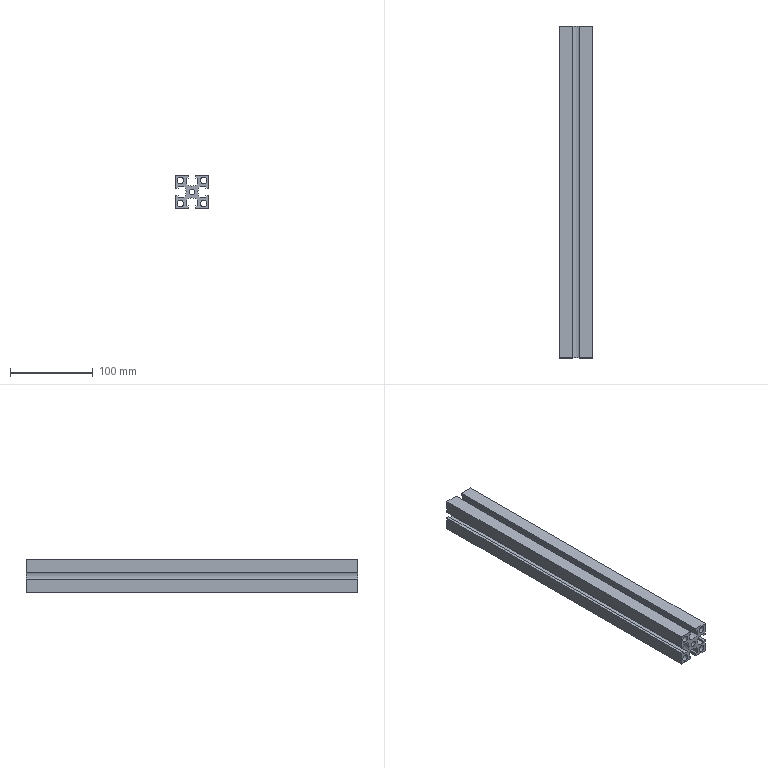Part | NX | 1 solid | 43 faces | box 40 x 400 x 40 mm | volume 318357 mm3 | plane 34 | cylinder 9 | commonest cylinder face diameters 8 x4 20 x4 6.8 x1
STEP:
#1=CARTESIAN_POINT('',(-236.,550.,-35.75));
#2=VERTEX_POINT('',#1);
#3=CARTESIAN_POINT('',(-236.,550.,-20.));
#4=VERTEX_POINT('',#3);
#5=CARTESIAN_POINT('',(-236.,550.,-35.75));
#6=DIRECTION('',(0.,0.,1.));
#7=VECTOR('',#6,1000.);
#8=LINE('',#5,#7);
#9=EDGE_CURVE('',#2,#4,#8,.T.);
#10=ORIENTED_EDGE('',*,*,#9,.T.);
#11=CARTESIAN_POINT('',(-236.,150.,-20.));
#12=VERTEX_POINT('',#11);
#13=CARTESIAN_POINT('',(-236.,150.,-20.));
#14=DIRECTION('',(0.,1.,0.));
#15=VECTOR('',#14,1000.);
#16=LINE('',#13,#15);
#17=EDGE_CURVE('',#12,#4,#16,.T.);
#18=ORIENTED_EDGE('',*,*,#17,.F.);
#19=CARTESIAN_POINT('',(-236.,150.,-35.75));
#20=VERTEX_POINT('',#19);
#21=CARTESIAN_POINT('',(-236.,150.,-35.75));
#22=DIRECTION('',(0.,0.,1.));
#23=VECTOR('',#22,1000.);
#24=LINE('',#21,#23);
#25=EDGE_CURVE('',#20,#12,#24,.T.);
#26=ORIENTED_EDGE('',*,*,#25,.F.);
#27=CARTESIAN_POINT('',(-236.,150.,-35.75));
#28=DIRECTION('',(0.,1.,0.));
#29=VECTOR('',#28,1000.);
#30=LINE('',#27,#29);
#31=EDGE_CURVE('',#20,#2,#30,.T.);
#32=ORIENTED_EDGE('',*,*,#31,.T.);
#33=EDGE_LOOP('',(#10,#18,#26,#32));
#34=FACE_BOUND('',#33,.T.);
#35=CARTESIAN_POINT('',(-236.,150.,-35.75));
#36=DIRECTION('',(-1.,0.,0.));
#37=DIRECTION('',(0.,0.,1.));
#38=AXIS2_PLACEMENT_3D('',#35,#36,#37);
#39=PLANE('',#38);
#40=ADVANCED_FACE('',(#34),#39,.F.);
#41=CARTESIAN_POINT('',(-251.75,550.,-20.));
#42=VERTEX_POINT('',#41);
#43=CARTESIAN_POINT('',(-236.,550.,-20.));
#44=DIRECTION('',(-1.,0.,0.));
#45=VECTOR('',#44,1000.);
#46=LINE('',#43,#45);
#47=EDGE_CURVE('',#4,#42,#46,.T.);
#48=ORIENTED_EDGE('',*,*,#47,.T.);
#49=CARTESIAN_POINT('',(-251.75,150.,-20.));
#50=VERTEX_POINT('',#49);
#51=CARTESIAN_POINT('',(-251.75,150.,-20.));
#52=DIRECTION('',(0.,1.,0.));
#53=VECTOR('',#52,1000.);
#54=LINE('',#51,#53);
#55=EDGE_CURVE('',#50,#42,#54,.T.);
#56=ORIENTED_EDGE('',*,*,#55,.F.);
#57=CARTESIAN_POINT('',(-236.,150.,-20.));
#58=DIRECTION('',(-1.,0.,0.));
#59=VECTOR('',#58,1000.);
#60=LINE('',#57,#59);
#61=EDGE_CURVE('',#12,#50,#60,.T.);
#62=ORIENTED_EDGE('',*,*,#61,.F.);
#63=ORIENTED_EDGE('',*,*,#17,.T.);
#64=EDGE_LOOP('',(#48,#56,#62,#63));
#65=FACE_BOUND('',#64,.T.);
#66=CARTESIAN_POINT('',(-236.,150.,-20.));
#67=DIRECTION('',(0.,0.,-1.));
#68=DIRECTION('',(-1.,0.,0.));
#69=AXIS2_PLACEMENT_3D('',#66,#67,#68);
#70=PLANE('',#69);
#71=ADVANCED_FACE('',(#65),#70,.F.);
#72=CARTESIAN_POINT('',(-251.75,550.,-23.5));
#73=VERTEX_POINT('',#72);
#74=CARTESIAN_POINT('',(-251.75,550.,-20.));
#75=DIRECTION('',(0.,0.,-1.));
#76=VECTOR('',#75,1000.);
#77=LINE('',#74,#76);
#78=EDGE_CURVE('',#42,#73,#77,.T.);
#79=ORIENTED_EDGE('',*,*,#78,.T.);
#80=CARTESIAN_POINT('',(-251.75,150.,-23.5));
#81=VERTEX_POINT('',#80);
#82=CARTESIAN_POINT('',(-251.75,150.,-23.5));
#83=DIRECTION('',(0.,1.,0.));
#84=VECTOR('',#83,1000.);
#85=LINE('',#82,#84);
#86=EDGE_CURVE('',#81,#73,#85,.T.);
#87=ORIENTED_EDGE('',*,*,#86,.F.);
#88=CARTESIAN_POINT('',(-251.75,150.,-20.));
#89=DIRECTION('',(0.,0.,-1.));
#90=VECTOR('',#89,1000.);
#91=LINE('',#88,#90);
#92=EDGE_CURVE('',#50,#81,#91,.T.);
#93=ORIENTED_EDGE('',*,*,#92,.F.);
#94=ORIENTED_EDGE('',*,*,#55,.T.);
#95=EDGE_LOOP('',(#79,#87,#93,#94));
#96=FACE_BOUND('',#95,.T.);
#97=CARTESIAN_POINT('',(-251.75,150.,-20.));
#98=DIRECTION('',(1.,0.,0.));
#99=DIRECTION('',(0.,0.,-1.));
#100=AXIS2_PLACEMENT_3D('',#97,#98,#99);
#101=PLANE('',#100);
#102=ADVANCED_FACE('',(#96),#101,.F.);
#103=CARTESIAN_POINT('',(-249.427,550.,-23.5));
#104=VERTEX_POINT('',#103);
#105=CARTESIAN_POINT('',(-251.75,550.,-23.5));
#106=DIRECTION('',(1.,0.,0.));
#107=VECTOR('',#106,1000.);
#108=LINE('',#105,#107);
#109=EDGE_CURVE('',#73,#104,#108,.T.);
#110=ORIENTED_EDGE('',*,*,#109,.T.);
#111=CARTESIAN_POINT('',(-249.427,150.,-23.5));
#112=VERTEX_POINT('',#111);
#113=CARTESIAN_POINT('',(-249.427,150.,-23.5));
#114=DIRECTION('',(0.,1.,0.));
#115=VECTOR('',#114,1000.);
#116=LINE('',#113,#115);
#117=EDGE_CURVE('',#112,#104,#116,.T.);
#118=ORIENTED_EDGE('',*,*,#117,.F.);
#119=CARTESIAN_POINT('',(-251.75,150.,-23.5));
#120=DIRECTION('',(1.,0.,0.));
#121=VECTOR('',#120,1000.);
#122=LINE('',#119,#121);
#123=EDGE_CURVE('',#81,#112,#122,.T.);
#124=ORIENTED_EDGE('',*,*,#123,.F.);
#125=ORIENTED_EDGE('',*,*,#86,.T.);
#126=EDGE_LOOP('',(#110,#118,#124,#125));
#127=FACE_BOUND('',#126,.T.);
#128=CARTESIAN_POINT('',(-251.75,150.,-23.5));
#129=DIRECTION('',(0.,0.,1.));
#130=DIRECTION('',(0.,-1.,0.));
#131=AXIS2_PLACEMENT_3D('',#128,#129,#130);
#132=PLANE('',#131);
#133=ADVANCED_FACE('',(#127),#132,.F.);
#134=CARTESIAN_POINT('',(-249.427,550.,-30.327));
#135=VERTEX_POINT('',#134);
#136=CARTESIAN_POINT('',(-249.427,550.,-23.5));
#137=DIRECTION('',(0.,0.,-1.));
#138=VECTOR('',#137,1000.);
#139=LINE('',#136,#138);
#140=EDGE_CURVE('',#104,#135,#139,.T.);
#141=ORIENTED_EDGE('',*,*,#140,.T.);
#142=CARTESIAN_POINT('',(-249.427,150.,-30.327));
#143=VERTEX_POINT('',#142);
#144=CARTESIAN_POINT('',(-249.427,150.,-30.327));
#145=DIRECTION('',(0.,1.,0.));
#146=VECTOR('',#145,1000.);
#147=LINE('',#144,#146);
#148=EDGE_CURVE('',#143,#135,#147,.T.);
#149=ORIENTED_EDGE('',*,*,#148,.F.);
#150=CARTESIAN_POINT('',(-249.427,150.,-23.5));
#151=DIRECTION('',(0.,0.,-1.));
#152=VECTOR('',#151,1000.);
#153=LINE('',#150,#152);
#154=EDGE_CURVE('',#112,#143,#153,.T.);
#155=ORIENTED_EDGE('',*,*,#154,.F.);
#156=ORIENTED_EDGE('',*,*,#117,.T.);
#157=EDGE_LOOP('',(#141,#149,#155,#156));
#158=FACE_BOUND('',#157,.T.);
#159=CARTESIAN_POINT('',(-249.427,150.,-23.5));
#160=DIRECTION('',(1.,0.,0.));
#161=DIRECTION('',(0.,0.,-1.));
#162=AXIS2_PLACEMENT_3D('',#159,#160,#161);
#163=PLANE('',#162);
#164=ADVANCED_FACE('',(#158),#163,.F.);
#165=CARTESIAN_POINT('',(-262.573,550.,-30.327));
#166=VERTEX_POINT('',#165);
#167=CARTESIAN_POINT('',(-256.,550.,-22.791));
#168=DIRECTION('',(0.,1.,0.));
#169=DIRECTION('',(-1.,0.,0.));
#170=AXIS2_PLACEMENT_3D('',#167,#168,#169);
#171=CIRCLE('',#170,10.);
#172=EDGE_CURVE('',#135,#166,#171,.T.);
#173=ORIENTED_EDGE('',*,*,#172,.T.);
#174=CARTESIAN_POINT('',(-262.573,150.,-30.327));
#175=VERTEX_POINT('',#174);
#176=CARTESIAN_POINT('',(-262.573,150.,-30.327));
#177=DIRECTION('',(0.,1.,0.));
#178=VECTOR('',#177,1000.);
#179=LINE('',#176,#178);
#180=EDGE_CURVE('',#175,#166,#179,.T.);
#181=ORIENTED_EDGE('',*,*,#180,.F.);
#182=CARTESIAN_POINT('',(-256.,150.,-22.791));
#183=DIRECTION('',(0.,1.,0.));
#184=DIRECTION('',(-1.,0.,0.));
#185=AXIS2_PLACEMENT_3D('',#182,#183,#184);
#186=CIRCLE('',#185,10.);
#187=EDGE_CURVE('',#143,#175,#186,.T.);
#188=ORIENTED_EDGE('',*,*,#187,.F.);
#189=ORIENTED_EDGE('',*,*,#148,.T.);
#190=EDGE_LOOP('',(#173,#181,#188,#189));
#191=FACE_BOUND('',#190,.T.);
#192=CARTESIAN_POINT('',(-256.,150.,-22.791));
#193=DIRECTION('',(0.,1.,0.));
#194=DIRECTION('',(0.,0.,1.));
#195=AXIS2_PLACEMENT_3D('',#192,#193,#194);
#196=CYLINDRICAL_SURFACE('',#195,10.);
#197=ADVANCED_FACE('',(#191),#196,.F.);
#198=CARTESIAN_POINT('',(-262.573,550.,-23.5));
#199=VERTEX_POINT('',#198);
#200=CARTESIAN_POINT('',(-262.573,550.,-30.327));
#201=DIRECTION('',(0.,0.,1.));
#202=VECTOR('',#201,1000.);
#203=LINE('',#200,#202);
#204=EDGE_CURVE('',#166,#199,#203,.T.);
#205=ORIENTED_EDGE('',*,*,#204,.T.);
#206=CARTESIAN_POINT('',(-262.573,150.,-23.5));
#207=VERTEX_POINT('',#206);
#208=CARTESIAN_POINT('',(-262.573,150.,-23.5));
#209=DIRECTION('',(0.,1.,0.));
#210=VECTOR('',#209,1000.);
#211=LINE('',#208,#210);
#212=EDGE_CURVE('',#207,#199,#211,.T.);
#213=ORIENTED_EDGE('',*,*,#212,.F.);
#214=CARTESIAN_POINT('',(-262.573,150.,-30.327));
#215=DIRECTION('',(0.,0.,1.));
#216=VECTOR('',#215,1000.);
#217=LINE('',#214,#216);
#218=EDGE_CURVE('',#175,#207,#217,.T.);
#219=ORIENTED_EDGE('',*,*,#218,.F.);
#220=ORIENTED_EDGE('',*,*,#180,.T.);
#221=EDGE_LOOP('',(#205,#213,#219,#220));
#222=FACE_BOUND('',#221,.T.);
#223=CARTESIAN_POINT('',(-262.573,150.,-30.327));
#224=DIRECTION('',(-1.,0.,0.));
#225=DIRECTION('',(0.,0.,1.));
#226=AXIS2_PLACEMENT_3D('',#223,#224,#225);
#227=PLANE('',#226);
#228=ADVANCED_FACE('',(#222),#227,.F.);
#229=CARTESIAN_POINT('',(-260.25,550.,-23.5));
#230=VERTEX_POINT('',#229);
#231=CARTESIAN_POINT('',(-262.573,550.,-23.5));
#232=DIRECTION('',(1.,0.,0.));
#233=VECTOR('',#232,1000.);
#234=LINE('',#231,#233);
#235=EDGE_CURVE('',#199,#230,#234,.T.);
#236=ORIENTED_EDGE('',*,*,#235,.T.);
#237=CARTESIAN_POINT('',(-260.25,150.,-23.5));
#238=VERTEX_POINT('',#237);
#239=CARTESIAN_POINT('',(-260.25,150.,-23.5));
#240=DIRECTION('',(0.,1.,0.));
#241=VECTOR('',#240,1000.);
#242=LINE('',#239,#241);
#243=EDGE_CURVE('',#238,#230,#242,.T.);
#244=ORIENTED_EDGE('',*,*,#243,.F.);
#245=CARTESIAN_POINT('',(-262.573,150.,-23.5));
#246=DIRECTION('',(1.,0.,0.));
#247=VECTOR('',#246,1000.);
#248=LINE('',#245,#247);
#249=EDGE_CURVE('',#207,#238,#248,.T.);
#250=ORIENTED_EDGE('',*,*,#249,.F.);
#251=ORIENTED_EDGE('',*,*,#212,.T.);
#252=EDGE_LOOP('',(#236,#244,#250,#251));
#253=FACE_BOUND('',#252,.T.);
#254=CARTESIAN_POINT('',(-262.573,150.,-23.5));
#255=DIRECTION('',(0.,0.,1.));
#256=DIRECTION('',(0.,-1.,0.));
#257=AXIS2_PLACEMENT_3D('',#254,#255,#256);
#258=PLANE('',#257);
#259=ADVANCED_FACE('',(#253),#258,.F.);
#260=CARTESIAN_POINT('',(-260.25,550.,-20.));
#261=VERTEX_POINT('',#260);
#262=CARTESIAN_POINT('',(-260.25,550.,-23.5));
#263=DIRECTION('',(0.,0.,1.));
#264=VECTOR('',#263,1000.);
#265=LINE('',#262,#264);
#266=EDGE_CURVE('',#230,#261,#265,.T.);
#267=ORIENTED_EDGE('',*,*,#266,.T.);
#268=CARTESIAN_POINT('',(-260.25,150.,-20.));
#269=VERTEX_POINT('',#268);
#270=CARTESIAN_POINT('',(-260.25,150.,-20.));
#271=DIRECTION('',(0.,1.,0.));
#272=VECTOR('',#271,1000.);
#273=LINE('',#270,#272);
#274=EDGE_CURVE('',#269,#261,#273,.T.);
#275=ORIENTED_EDGE('',*,*,#274,.F.);
#276=CARTESIAN_POINT('',(-260.25,150.,-23.5));
#277=DIRECTION('',(0.,0.,1.));
#278=VECTOR('',#277,1000.);
#279=LINE('',#276,#278);
#280=EDGE_CURVE('',#238,#269,#279,.T.);
#281=ORIENTED_EDGE('',*,*,#280,.F.);
#282=ORIENTED_EDGE('',*,*,#243,.T.);
#283=EDGE_LOOP('',(#267,#275,#281,#282));
#284=FACE_BOUND('',#283,.T.);
#285=CARTESIAN_POINT('',(-260.25,150.,-23.5));
#286=DIRECTION('',(-1.,0.,0.));
#287=DIRECTION('',(0.,0.,1.));
#288=AXIS2_PLACEMENT_3D('',#285,#286,#287);
#289=PLANE('',#288);
#290=ADVANCED_FACE('',(#284),#289,.F.);
#291=CARTESIAN_POINT('',(-276.,550.,-20.));
#292=VERTEX_POINT('',#291);
#293=CARTESIAN_POINT('',(-260.25,550.,-20.));
#294=DIRECTION('',(-1.,0.,0.));
#295=VECTOR('',#294,1000.);
#296=LINE('',#293,#295);
#297=EDGE_CURVE('',#261,#292,#296,.T.);
#298=ORIENTED_EDGE('',*,*,#297,.T.);
#299=CARTESIAN_POINT('',(-276.,150.,-20.));
#300=VERTEX_POINT('',#299);
#301=CARTESIAN_POINT('',(-276.,150.,-20.));
#302=DIRECTION('',(0.,1.,0.));
#303=VECTOR('',#302,1000.);
#304=LINE('',#301,#303);
#305=EDGE_CURVE('',#300,#292,#304,.T.);
#306=ORIENTED_EDGE('',*,*,#305,.F.);
#307=CARTESIAN_POINT('',(-260.25,150.,-20.));
#308=DIRECTION('',(-1.,0.,0.));
#309=VECTOR('',#308,1000.);
#310=LINE('',#307,#309);
#311=EDGE_CURVE('',#269,#300,#310,.T.);
#312=ORIENTED_EDGE('',*,*,#311,.F.);
#313=ORIENTED_EDGE('',*,*,#274,.T.);
#314=EDGE_LOOP('',(#298,#306,#312,#313));
#315=FACE_BOUND('',#314,.T.);
#316=CARTESIAN_POINT('',(-260.25,150.,-20.));
#317=DIRECTION('',(0.,0.,-1.));
#318=DIRECTION('',(-1.,0.,0.));
#319=AXIS2_PLACEMENT_3D('',#316,#317,#318);
#320=PLANE('',#319);
#321=ADVANCED_FACE('',(#315),#320,.F.);
#322=CARTESIAN_POINT('',(-276.,550.,-35.75));
#323=VERTEX_POINT('',#322);
#324=CARTESIAN_POINT('',(-276.,550.,-20.));
#325=DIRECTION('',(0.,0.,-1.));
#326=VECTOR('',#325,1000.);
#327=LINE('',#324,#326);
#328=EDGE_CURVE('',#292,#323,#327,.T.);
#329=ORIENTED_EDGE('',*,*,#328,.T.);
#330=CARTESIAN_POINT('',(-276.,150.,-35.75));
#331=VERTEX_POINT('',#330);
#332=CARTESIAN_POINT('',(-276.,150.,-35.75));
#333=DIRECTION('',(0.,1.,0.));
#334=VECTOR('',#333,1000.);
#335=LINE('',#332,#334);
#336=EDGE_CURVE('',#331,#323,#335,.T.);
#337=ORIENTED_EDGE('',*,*,#336,.F.);
#338=CARTESIAN_POINT('',(-276.,150.,-20.));
#339=DIRECTION('',(0.,0.,-1.));
#340=VECTOR('',#339,1000.);
#341=LINE('',#338,#340);
#342=EDGE_CURVE('',#300,#331,#341,.T.);
#343=ORIENTED_EDGE('',*,*,#342,.F.);
#344=ORIENTED_EDGE('',*,*,#305,.T.);
#345=EDGE_LOOP('',(#329,#337,#343,#344));
#346=FACE_BOUND('',#345,.T.);
#347=CARTESIAN_POINT('',(-276.,150.,-20.));
#348=DIRECTION('',(1.,0.,0.));
#349=DIRECTION('',(0.,0.,-1.));
#350=AXIS2_PLACEMENT_3D('',#347,#348,#349);
#351=PLANE('',#350);
#352=ADVANCED_FACE('',(#346),#351,.F.);
#353=CARTESIAN_POINT('',(-272.5,550.,-35.75));
#354=VERTEX_POINT('',#353);
#355=CARTESIAN_POINT('',(-276.,550.,-35.75));
#356=DIRECTION('',(1.,0.,0.));
#357=VECTOR('',#356,1000.);
#358=LINE('',#355,#357);
#359=EDGE_CURVE('',#323,#354,#358,.T.);
#360=ORIENTED_EDGE('',*,*,#359,.T.);
#361=CARTESIAN_POINT('',(-272.5,150.,-35.75));
#362=VERTEX_POINT('',#361);
#363=CARTESIAN_POINT('',(-272.5,150.,-35.75));
#364=DIRECTION('',(0.,1.,0.));
#365=VECTOR('',#364,1000.);
#366=LINE('',#363,#365);
#367=EDGE_CURVE('',#362,#354,#366,.T.);
#368=ORIENTED_EDGE('',*,*,#367,.F.);
#369=CARTESIAN_POINT('',(-276.,150.,-35.75));
#370=DIRECTION('',(1.,0.,0.));
#371=VECTOR('',#370,1000.);
#372=LINE('',#369,#371);
#373=EDGE_CURVE('',#331,#362,#372,.T.);
#374=ORIENTED_EDGE('',*,*,#373,.F.);
#375=ORIENTED_EDGE('',*,*,#336,.T.);
#376=EDGE_LOOP('',(#360,#368,#374,#375));
#377=FACE_BOUND('',#376,.T.);
#378=CARTESIAN_POINT('',(-276.,150.,-35.75));
#379=DIRECTION('',(0.,0.,1.));
#380=DIRECTION('',(1.,0.,0.));
#381=AXIS2_PLACEMENT_3D('',#378,#379,#380);
#382=PLANE('',#381);
#383=ADVANCED_FACE('',(#377),#382,.F.);
#384=CARTESIAN_POINT('',(-272.5,550.,-33.427));
#385=VERTEX_POINT('',#384);
#386=CARTESIAN_POINT('',(-272.5,550.,-35.75));
#387=DIRECTION('',(0.,0.,1.));
#388=VECTOR('',#387,1000.);
#389=LINE('',#386,#388);
#390=EDGE_CURVE('',#354,#385,#389,.T.);
#391=ORIENTED_EDGE('',*,*,#390,.T.);
#392=CARTESIAN_POINT('',(-272.5,150.,-33.427));
#393=VERTEX_POINT('',#392);
#394=CARTESIAN_POINT('',(-272.5,150.,-33.427));
#395=DIRECTION('',(0.,1.,0.));
#396=VECTOR('',#395,1000.);
#397=LINE('',#394,#396);
#398=EDGE_CURVE('',#393,#385,#397,.T.);
#399=ORIENTED_EDGE('',*,*,#398,.F.);
#400=CARTESIAN_POINT('',(-272.5,150.,-35.75));
#401=DIRECTION('',(0.,0.,1.));
#402=VECTOR('',#401,1000.);
#403=LINE('',#400,#402);
#404=EDGE_CURVE('',#362,#393,#403,.T.);
#405=ORIENTED_EDGE('',*,*,#404,.F.);
#406=ORIENTED_EDGE('',*,*,#367,.T.);
#407=EDGE_LOOP('',(#391,#399,#405,#406));
#408=FACE_BOUND('',#407,.T.);
#409=CARTESIAN_POINT('',(-272.5,150.,-35.75));
#410=DIRECTION('',(-1.,0.,0.));
#411=DIRECTION('',(0.,0.,1.));
#412=AXIS2_PLACEMENT_3D('',#409,#410,#411);
#413=PLANE('',#412);
#414=ADVANCED_FACE('',(#408),#413,.F.);
#415=CARTESIAN_POINT('',(-265.673,550.,-33.427));
#416=VERTEX_POINT('',#415);
#417=CARTESIAN_POINT('',(-272.5,550.,-33.427));
#418=DIRECTION('',(1.,0.,0.));
#419=VECTOR('',#418,1000.);
#420=LINE('',#417,#419);
#421=EDGE_CURVE('',#385,#416,#420,.T.);
#422=ORIENTED_EDGE('',*,*,#421,.T.);
#423=CARTESIAN_POINT('',(-265.673,150.,-33.427));
#424=VERTEX_POINT('',#423);
#425=CARTESIAN_POINT('',(-265.673,150.,-33.427));
#426=DIRECTION('',(0.,1.,0.));
#427=VECTOR('',#426,1000.);
#428=LINE('',#425,#427);
#429=EDGE_CURVE('',#424,#416,#428,.T.);
#430=ORIENTED_EDGE('',*,*,#429,.F.);
#431=CARTESIAN_POINT('',(-272.5,150.,-33.427));
#432=DIRECTION('',(1.,0.,0.));
#433=VECTOR('',#432,1000.);
#434=LINE('',#431,#433);
#435=EDGE_CURVE('',#393,#424,#434,.T.);
#436=ORIENTED_EDGE('',*,*,#435,.F.);
#437=ORIENTED_EDGE('',*,*,#398,.T.);
#438=EDGE_LOOP('',(#422,#430,#436,#437));
#439=FACE_BOUND('',#438,.T.);
#440=CARTESIAN_POINT('',(-272.5,150.,-33.427));
#441=DIRECTION('',(0.,0.,1.));
#442=DIRECTION('',(1.,0.,0.));
#443=AXIS2_PLACEMENT_3D('',#440,#441,#442);
#444=PLANE('',#443);
#445=ADVANCED_FACE('',(#439),#444,.F.);
#446=CARTESIAN_POINT('',(-265.673,550.,-46.573));
#447=VERTEX_POINT('',#446);
#448=CARTESIAN_POINT('',(-273.209,550.,-40.));
#449=DIRECTION('',(0.,1.,0.));
#450=DIRECTION('',(-1.,0.,0.));
#451=AXIS2_PLACEMENT_3D('',#448,#449,#450);
#452=CIRCLE('',#451,10.);
#453=EDGE_CURVE('',#416,#447,#452,.T.);
#454=ORIENTED_EDGE('',*,*,#453,.T.);
#455=CARTESIAN_POINT('',(-265.673,150.,-46.573));
#456=VERTEX_POINT('',#455);
#457=CARTESIAN_POINT('',(-265.673,150.,-46.573));
#458=DIRECTION('',(0.,1.,0.));
#459=VECTOR('',#458,1000.);
#460=LINE('',#457,#459);
#461=EDGE_CURVE('',#456,#447,#460,.T.);
#462=ORIENTED_EDGE('',*,*,#461,.F.);
#463=CARTESIAN_POINT('',(-273.209,150.,-40.));
#464=DIRECTION('',(0.,1.,0.));
#465=DIRECTION('',(-1.,0.,0.));
#466=AXIS2_PLACEMENT_3D('',#463,#464,#465);
#467=CIRCLE('',#466,10.);
#468=EDGE_CURVE('',#424,#456,#467,.T.);
#469=ORIENTED_EDGE('',*,*,#468,.F.);
#470=ORIENTED_EDGE('',*,*,#429,.T.);
#471=EDGE_LOOP('',(#454,#462,#469,#470));
#472=FACE_BOUND('',#471,.T.);
#473=CARTESIAN_POINT('',(-273.209,150.,-40.));
#474=DIRECTION('',(0.,1.,0.));
#475=DIRECTION('',(0.,0.,1.));
#476=AXIS2_PLACEMENT_3D('',#473,#474,#475);
#477=CYLINDRICAL_SURFACE('',#476,10.);
#478=ADVANCED_FACE('',(#472),#477,.F.);
#479=CARTESIAN_POINT('',(-272.5,550.,-46.573));
#480=VERTEX_POINT('',#479);
#481=CARTESIAN_POINT('',(-265.673,550.,-46.573));
#482=DIRECTION('',(-1.,0.,0.));
#483=VECTOR('',#482,1000.);
#484=LINE('',#481,#483);
#485=EDGE_CURVE('',#447,#480,#484,.T.);
#486=ORIENTED_EDGE('',*,*,#485,.T.);
#487=CARTESIAN_POINT('',(-272.5,150.,-46.573));
#488=VERTEX_POINT('',#487);
#489=CARTESIAN_POINT('',(-272.5,150.,-46.573));
#490=DIRECTION('',(0.,1.,0.));
#491=VECTOR('',#490,1000.);
#492=LINE('',#489,#491);
#493=EDGE_CURVE('',#488,#480,#492,.T.);
#494=ORIENTED_EDGE('',*,*,#493,.F.);
#495=CARTESIAN_POINT('',(-265.673,150.,-46.573));
#496=DIRECTION('',(-1.,0.,0.));
#497=VECTOR('',#496,1000.);
#498=LINE('',#495,#497);
#499=EDGE_CURVE('',#456,#488,#498,.T.);
#500=ORIENTED_EDGE('',*,*,#499,.F.);
#501=ORIENTED_EDGE('',*,*,#461,.T.);
#502=EDGE_LOOP('',(#486,#494,#500,#501));
#503=FACE_BOUND('',#502,.T.);
#504=CARTESIAN_POINT('',(-265.673,150.,-46.573));
#505=DIRECTION('',(0.,0.,-1.));
#506=DIRECTION('',(-1.,0.,0.));
#507=AXIS2_PLACEMENT_3D('',#504,#505,#506);
#508=PLANE('',#507);
#509=ADVANCED_FACE('',(#503),#508,.F.);
#510=CARTESIAN_POINT('',(-272.5,550.,-44.25));
#511=VERTEX_POINT('',#510);
#512=CARTESIAN_POINT('',(-272.5,550.,-46.573));
#513=DIRECTION('',(0.,0.,1.));
#514=VECTOR('',#513,1000.);
#515=LINE('',#512,#514);
#516=EDGE_CURVE('',#480,#511,#515,.T.);
#517=ORIENTED_EDGE('',*,*,#516,.T.);
#518=CARTESIAN_POINT('',(-272.5,150.,-44.25));
#519=VERTEX_POINT('',#518);
#520=CARTESIAN_POINT('',(-272.5,150.,-44.25));
#521=DIRECTION('',(0.,1.,0.));
#522=VECTOR('',#521,1000.);
#523=LINE('',#520,#522);
#524=EDGE_CURVE('',#519,#511,#523,.T.);
#525=ORIENTED_EDGE('',*,*,#524,.F.);
#526=CARTESIAN_POINT('',(-272.5,150.,-46.573));
#527=DIRECTION('',(0.,0.,1.));
#528=VECTOR('',#527,1000.);
#529=LINE('',#526,#528);
#530=EDGE_CURVE('',#488,#519,#529,.T.);
#531=ORIENTED_EDGE('',*,*,#530,.F.);
#532=ORIENTED_EDGE('',*,*,#493,.T.);
#533=EDGE_LOOP('',(#517,#525,#531,#532));
#534=FACE_BOUND('',#533,.T.);
#535=CARTESIAN_POINT('',(-272.5,150.,-46.573));
#536=DIRECTION('',(-1.,0.,0.));
#537=DIRECTION('',(0.,0.,1.));
#538=AXIS2_PLACEMENT_3D('',#535,#536,#537);
#539=PLANE('',#538);
#540=ADVANCED_FACE('',(#534),#539,.F.);
#541=CARTESIAN_POINT('',(-276.,550.,-44.25));
#542=VERTEX_POINT('',#541);
#543=CARTESIAN_POINT('',(-272.5,550.,-44.25));
#544=DIRECTION('',(-1.,0.,0.));
#545=VECTOR('',#544,1000.);
#546=LINE('',#543,#545);
#547=EDGE_CURVE('',#511,#542,#546,.T.);
#548=ORIENTED_EDGE('',*,*,#547,.T.);
#549=CARTESIAN_POINT('',(-276.,150.,-44.25));
#550=VERTEX_POINT('',#549);
#551=CARTESIAN_POINT('',(-276.,150.,-44.25));
#552=DIRECTION('',(0.,1.,0.));
#553=VECTOR('',#552,1000.);
#554=LINE('',#551,#553);
#555=EDGE_CURVE('',#550,#542,#554,.T.);
#556=ORIENTED_EDGE('',*,*,#555,.F.);
#557=CARTESIAN_POINT('',(-272.5,150.,-44.25));
#558=DIRECTION('',(-1.,0.,0.));
#559=VECTOR('',#558,1000.);
#560=LINE('',#557,#559);
#561=EDGE_CURVE('',#519,#550,#560,.T.);
#562=ORIENTED_EDGE('',*,*,#561,.F.);
#563=ORIENTED_EDGE('',*,*,#524,.T.);
#564=EDGE_LOOP('',(#548,#556,#562,#563));
#565=FACE_BOUND('',#564,.T.);
#566=CARTESIAN_POINT('',(-272.5,150.,-44.25));
#567=DIRECTION('',(0.,0.,-1.));
#568=DIRECTION('',(-1.,0.,0.));
#569=AXIS2_PLACEMENT_3D('',#566,#567,#568);
#570=PLANE('',#569);
#571=ADVANCED_FACE('',(#565),#570,.F.);
#572=CARTESIAN_POINT('',(-276.,550.,-60.));
#573=VERTEX_POINT('',#572);
#574=CARTESIAN_POINT('',(-276.,550.,-44.25));
#575=DIRECTION('',(0.,0.,-1.));
#576=VECTOR('',#575,1000.);
#577=LINE('',#574,#576);
#578=EDGE_CURVE('',#542,#573,#577,.T.);
#579=ORIENTED_EDGE('',*,*,#578,.T.);
#580=CARTESIAN_POINT('',(-276.,150.,-60.));
#581=VERTEX_POINT('',#580);
#582=CARTESIAN_POINT('',(-276.,150.,-60.));
#583=DIRECTION('',(0.,1.,0.));
#584=VECTOR('',#583,1000.);
#585=LINE('',#582,#584);
#586=EDGE_CURVE('',#581,#573,#585,.T.);
#587=ORIENTED_EDGE('',*,*,#586,.F.);
#588=CARTESIAN_POINT('',(-276.,150.,-44.25));
#589=DIRECTION('',(0.,0.,-1.));
#590=VECTOR('',#589,1000.);
#591=LINE('',#588,#590);
#592=EDGE_CURVE('',#550,#581,#591,.T.);
#593=ORIENTED_EDGE('',*,*,#592,.F.);
#594=ORIENTED_EDGE('',*,*,#555,.T.);
#595=EDGE_LOOP('',(#579,#587,#593,#594));
#596=FACE_BOUND('',#595,.T.);
#597=CARTESIAN_POINT('',(-276.,150.,-44.25));
#598=DIRECTION('',(1.,0.,0.));
#599=DIRECTION('',(0.,0.,-1.));
#600=AXIS2_PLACEMENT_3D('',#597,#598,#599);
#601=PLANE('',#600);
#602=ADVANCED_FACE('',(#596),#601,.F.);
#603=CARTESIAN_POINT('',(-260.25,550.,-60.));
#604=VERTEX_POINT('',#603);
#605=CARTESIAN_POINT('',(-276.,550.,-60.));
#606=DIRECTION('',(1.,0.,0.));
#607=VECTOR('',#606,1000.);
#608=LINE('',#605,#607);
#609=EDGE_CURVE('',#573,#604,#608,.T.);
#610=ORIENTED_EDGE('',*,*,#609,.T.);
#611=CARTESIAN_POINT('',(-260.25,150.,-60.));
#612=VERTEX_POINT('',#611);
#613=CARTESIAN_POINT('',(-260.25,150.,-60.));
#614=DIRECTION('',(0.,1.,0.));
#615=VECTOR('',#614,1000.);
#616=LINE('',#613,#615);
#617=EDGE_CURVE('',#612,#604,#616,.T.);
#618=ORIENTED_EDGE('',*,*,#617,.F.);
#619=CARTESIAN_POINT('',(-276.,150.,-60.));
#620=DIRECTION('',(1.,0.,0.));
#621=VECTOR('',#620,1000.);
#622=LINE('',#619,#621);
#623=EDGE_CURVE('',#581,#612,#622,.T.);
#624=ORIENTED_EDGE('',*,*,#623,.F.);
#625=ORIENTED_EDGE('',*,*,#586,.T.);
#626=EDGE_LOOP('',(#610,#618,#624,#625));
#627=FACE_BOUND('',#626,.T.);
#628=CARTESIAN_POINT('',(-276.,150.,-60.));
#629=DIRECTION('',(0.,0.,1.));
#630=DIRECTION('',(0.,-1.,0.));
#631=AXIS2_PLACEMENT_3D('',#628,#629,#630);
#632=PLANE('',#631);
#633=ADVANCED_FACE('',(#627),#632,.F.);
#634=CARTESIAN_POINT('',(-260.25,550.,-56.5));
#635=VERTEX_POINT('',#634);
#636=CARTESIAN_POINT('',(-260.25,550.,-60.));
#637=DIRECTION('',(0.,0.,1.));
#638=VECTOR('',#637,1000.);
#639=LINE('',#636,#638);
#640=EDGE_CURVE('',#604,#635,#639,.T.);
#641=ORIENTED_EDGE('',*,*,#640,.T.);
#642=CARTESIAN_POINT('',(-260.25,150.,-56.5));
#643=VERTEX_POINT('',#642);
#644=CARTESIAN_POINT('',(-260.25,150.,-56.5));
#645=DIRECTION('',(0.,1.,0.));
#646=VECTOR('',#645,1000.);
#647=LINE('',#644,#646);
#648=EDGE_CURVE('',#643,#635,#647,.T.);
#649=ORIENTED_EDGE('',*,*,#648,.F.);
#650=CARTESIAN_POINT('',(-260.25,150.,-60.));
#651=DIRECTION('',(0.,0.,1.));
#652=VECTOR('',#651,1000.);
#653=LINE('',#650,#652);
#654=EDGE_CURVE('',#612,#643,#653,.T.);
#655=ORIENTED_EDGE('',*,*,#654,.F.);
#656=ORIENTED_EDGE('',*,*,#617,.T.);
#657=EDGE_LOOP('',(#641,#649,#655,#656));
#658=FACE_BOUND('',#657,.T.);
#659=CARTESIAN_POINT('',(-260.25,150.,-60.));
#660=DIRECTION('',(-1.,0.,0.));
#661=DIRECTION('',(0.,0.,1.));
#662=AXIS2_PLACEMENT_3D('',#659,#660,#661);
#663=PLANE('',#662);
#664=ADVANCED_FACE('',(#658),#663,.F.);
#665=CARTESIAN_POINT('',(-262.573,550.,-56.5));
#666=VERTEX_POINT('',#665);
#667=CARTESIAN_POINT('',(-260.25,550.,-56.5));
#668=DIRECTION('',(-1.,0.,0.));
#669=VECTOR('',#668,1000.);
#670=LINE('',#667,#669);
#671=EDGE_CURVE('',#635,#666,#670,.T.);
#672=ORIENTED_EDGE('',*,*,#671,.T.);
#673=CARTESIAN_POINT('',(-262.573,150.,-56.5));
#674=VERTEX_POINT('',#673);
#675=CARTESIAN_POINT('',(-262.573,150.,-56.5));
#676=DIRECTION('',(0.,1.,0.));
#677=VECTOR('',#676,1000.);
#678=LINE('',#675,#677);
#679=EDGE_CURVE('',#674,#666,#678,.T.);
#680=ORIENTED_EDGE('',*,*,#679,.F.);
#681=CARTESIAN_POINT('',(-260.25,150.,-56.5));
#682=DIRECTION('',(-1.,0.,0.));
#683=VECTOR('',#682,1000.);
#684=LINE('',#681,#683);
#685=EDGE_CURVE('',#643,#674,#684,.T.);
#686=ORIENTED_EDGE('',*,*,#685,.F.);
#687=ORIENTED_EDGE('',*,*,#648,.T.);
#688=EDGE_LOOP('',(#672,#680,#686,#687));
#689=FACE_BOUND('',#688,.T.);
#690=CARTESIAN_POINT('',(-260.25,150.,-56.5));
#691=DIRECTION('',(0.,0.,-1.));
#692=DIRECTION('',(-1.,0.,0.));
#693=AXIS2_PLACEMENT_3D('',#690,#691,#692);
#694=PLANE('',#693);
#695=ADVANCED_FACE('',(#689),#694,.F.);
#696=CARTESIAN_POINT('',(-262.573,550.,-49.673));
#697=VERTEX_POINT('',#696);
#698=CARTESIAN_POINT('',(-262.573,550.,-56.5));
#699=DIRECTION('',(0.,0.,1.));
#700=VECTOR('',#699,1000.);
#701=LINE('',#698,#700);
#702=EDGE_CURVE('',#666,#697,#701,.T.);
#703=ORIENTED_EDGE('',*,*,#702,.T.);
#704=CARTESIAN_POINT('',(-262.573,150.,-49.673));
#705=VERTEX_POINT('',#704);
#706=CARTESIAN_POINT('',(-262.573,150.,-49.673));
#707=DIRECTION('',(0.,1.,0.));
#708=VECTOR('',#707,1000.);
#709=LINE('',#706,#708);
#710=EDGE_CURVE('',#705,#697,#709,.T.);
#711=ORIENTED_EDGE('',*,*,#710,.F.);
#712=CARTESIAN_POINT('',(-262.573,150.,-56.5));
#713=DIRECTION('',(0.,0.,1.));
#714=VECTOR('',#713,1000.);
#715=LINE('',#712,#714);
#716=EDGE_CURVE('',#674,#705,#715,.T.);
#717=ORIENTED_EDGE('',*,*,#716,.F.);
#718=ORIENTED_EDGE('',*,*,#679,.T.);
#719=EDGE_LOOP('',(#703,#711,#717,#718));
#720=FACE_BOUND('',#719,.T.);
#721=CARTESIAN_POINT('',(-262.573,150.,-56.5));
#722=DIRECTION('',(-1.,0.,0.));
#723=DIRECTION('',(0.,0.,1.));
#724=AXIS2_PLACEMENT_3D('',#721,#722,#723);
#725=PLANE('',#724);
#726=ADVANCED_FACE('',(#720),#725,.F.);
#727=CARTESIAN_POINT('',(-249.427,550.,-49.673));
#728=VERTEX_POINT('',#727);
#729=CARTESIAN_POINT('',(-256.,550.,-57.209));
#730=DIRECTION('',(0.,1.,0.));
#731=DIRECTION('',(-1.,0.,0.));
#732=AXIS2_PLACEMENT_3D('',#729,#730,#731);
#733=CIRCLE('',#732,10.);
#734=EDGE_CURVE('',#697,#728,#733,.T.);
#735=ORIENTED_EDGE('',*,*,#734,.T.);
#736=CARTESIAN_POINT('',(-249.427,150.,-49.673));
#737=VERTEX_POINT('',#736);
#738=CARTESIAN_POINT('',(-249.427,150.,-49.673));
#739=DIRECTION('',(0.,1.,0.));
#740=VECTOR('',#739,1000.);
#741=LINE('',#738,#740);
#742=EDGE_CURVE('',#737,#728,#741,.T.);
#743=ORIENTED_EDGE('',*,*,#742,.F.);
#744=CARTESIAN_POINT('',(-256.,150.,-57.209));
#745=DIRECTION('',(0.,1.,0.));
#746=DIRECTION('',(-1.,0.,0.));
#747=AXIS2_PLACEMENT_3D('',#744,#745,#746);
#748=CIRCLE('',#747,10.);
#749=EDGE_CURVE('',#705,#737,#748,.T.);
#750=ORIENTED_EDGE('',*,*,#749,.F.);
#751=ORIENTED_EDGE('',*,*,#710,.T.);
#752=EDGE_LOOP('',(#735,#743,#750,#751));
#753=FACE_BOUND('',#752,.T.);
#754=CARTESIAN_POINT('',(-256.,150.,-57.209));
#755=DIRECTION('',(0.,1.,0.));
#756=DIRECTION('',(0.,0.,1.));
#757=AXIS2_PLACEMENT_3D('',#754,#755,#756);
#758=CYLINDRICAL_SURFACE('',#757,10.);
#759=ADVANCED_FACE('',(#753),#758,.F.);
#760=CARTESIAN_POINT('',(-249.427,550.,-56.5));
#761=VERTEX_POINT('',#760);
#762=CARTESIAN_POINT('',(-249.427,550.,-49.673));
#763=DIRECTION('',(0.,0.,-1.));
#764=VECTOR('',#763,1000.);
#765=LINE('',#762,#764);
#766=EDGE_CURVE('',#728,#761,#765,.T.);
#767=ORIENTED_EDGE('',*,*,#766,.T.);
#768=CARTESIAN_POINT('',(-249.427,150.,-56.5));
#769=VERTEX_POINT('',#768);
#770=CARTESIAN_POINT('',(-249.427,150.,-56.5));
#771=DIRECTION('',(0.,1.,0.));
#772=VECTOR('',#771,1000.);
#773=LINE('',#770,#772);
#774=EDGE_CURVE('',#769,#761,#773,.T.);
#775=ORIENTED_EDGE('',*,*,#774,.F.);
#776=CARTESIAN_POINT('',(-249.427,150.,-49.673));
#777=DIRECTION('',(0.,0.,-1.));
#778=VECTOR('',#777,1000.);
#779=LINE('',#776,#778);
#780=EDGE_CURVE('',#737,#769,#779,.T.);
#781=ORIENTED_EDGE('',*,*,#780,.F.);
#782=ORIENTED_EDGE('',*,*,#742,.T.);
#783=EDGE_LOOP('',(#767,#775,#781,#782));
#784=FACE_BOUND('',#783,.T.);
#785=CARTESIAN_POINT('',(-249.427,150.,-49.673));
#786=DIRECTION('',(1.,0.,0.));
#787=DIRECTION('',(0.,0.,-1.));
#788=AXIS2_PLACEMENT_3D('',#785,#786,#787);
#789=PLANE('',#788);
#790=ADVANCED_FACE('',(#784),#789,.F.);
#791=CARTESIAN_POINT('',(-251.75,550.,-56.5));
#792=VERTEX_POINT('',#791);
#793=CARTESIAN_POINT('',(-249.427,550.,-56.5));
#794=DIRECTION('',(-1.,0.,0.));
#795=VECTOR('',#794,1000.);
#796=LINE('',#793,#795);
#797=EDGE_CURVE('',#761,#792,#796,.T.);
#798=ORIENTED_EDGE('',*,*,#797,.T.);
#799=CARTESIAN_POINT('',(-251.75,150.,-56.5));
#800=VERTEX_POINT('',#799);
#801=CARTESIAN_POINT('',(-251.75,150.,-56.5));
#802=DIRECTION('',(0.,1.,0.));
#803=VECTOR('',#802,1000.);
#804=LINE('',#801,#803);
#805=EDGE_CURVE('',#800,#792,#804,.T.);
#806=ORIENTED_EDGE('',*,*,#805,.F.);
#807=CARTESIAN_POINT('',(-249.427,150.,-56.5));
#808=DIRECTION('',(-1.,0.,0.));
#809=VECTOR('',#808,1000.);
#810=LINE('',#807,#809);
#811=EDGE_CURVE('',#769,#800,#810,.T.);
#812=ORIENTED_EDGE('',*,*,#811,.F.);
#813=ORIENTED_EDGE('',*,*,#774,.T.);
#814=EDGE_LOOP('',(#798,#806,#812,#813));
#815=FACE_BOUND('',#814,.T.);
#816=CARTESIAN_POINT('',(-249.427,150.,-56.5));
#817=DIRECTION('',(0.,0.,-1.));
#818=DIRECTION('',(-1.,0.,0.));
#819=AXIS2_PLACEMENT_3D('',#816,#817,#818);
#820=PLANE('',#819);
#821=ADVANCED_FACE('',(#815),#820,.F.);
#822=CARTESIAN_POINT('',(-251.75,550.,-60.));
#823=VERTEX_POINT('',#822);
#824=CARTESIAN_POINT('',(-251.75,550.,-56.5));
#825=DIRECTION('',(0.,0.,-1.));
#826=VECTOR('',#825,1000.);
#827=LINE('',#824,#826);
#828=EDGE_CURVE('',#792,#823,#827,.T.);
#829=ORIENTED_EDGE('',*,*,#828,.T.);
#830=CARTESIAN_POINT('',(-251.75,150.,-60.));
#831=VERTEX_POINT('',#830);
#832=CARTESIAN_POINT('',(-251.75,150.,-60.));
#833=DIRECTION('',(0.,1.,0.));
#834=VECTOR('',#833,1000.);
#835=LINE('',#832,#834);
#836=EDGE_CURVE('',#831,#823,#835,.T.);
#837=ORIENTED_EDGE('',*,*,#836,.F.);
#838=CARTESIAN_POINT('',(-251.75,150.,-56.5));
#839=DIRECTION('',(0.,0.,-1.));
#840=VECTOR('',#839,1000.);
#841=LINE('',#838,#840);
#842=EDGE_CURVE('',#800,#831,#841,.T.);
#843=ORIENTED_EDGE('',*,*,#842,.F.);
#844=ORIENTED_EDGE('',*,*,#805,.T.);
#845=EDGE_LOOP('',(#829,#837,#843,#844));
#846=FACE_BOUND('',#845,.T.);
#847=CARTESIAN_POINT('',(-251.75,150.,-56.5));
#848=DIRECTION('',(1.,0.,0.));
#849=DIRECTION('',(0.,0.,-1.));
#850=AXIS2_PLACEMENT_3D('',#847,#848,#849);
#851=PLANE('',#850);
#852=ADVANCED_FACE('',(#846),#851,.F.);
#853=CARTESIAN_POINT('',(-236.,550.,-60.));
#854=VERTEX_POINT('',#853);
#855=CARTESIAN_POINT('',(-251.75,550.,-60.));
#856=DIRECTION('',(1.,0.,0.));
#857=VECTOR('',#856,1000.);
#858=LINE('',#855,#857);
#859=EDGE_CURVE('',#823,#854,#858,.T.);
#860=ORIENTED_EDGE('',*,*,#859,.T.);
#861=CARTESIAN_POINT('',(-236.,150.,-60.));
#862=VERTEX_POINT('',#861);
#863=CARTESIAN_POINT('',(-236.,150.,-60.));
#864=DIRECTION('',(0.,1.,0.));
#865=VECTOR('',#864,1000.);
#866=LINE('',#863,#865);
#867=EDGE_CURVE('',#862,#854,#866,.T.);
#868=ORIENTED_EDGE('',*,*,#867,.F.);
#869=CARTESIAN_POINT('',(-251.75,150.,-60.));
#870=DIRECTION('',(1.,0.,0.));
#871=VECTOR('',#870,1000.);
#872=LINE('',#869,#871);
#873=EDGE_CURVE('',#831,#862,#872,.T.);
#874=ORIENTED_EDGE('',*,*,#873,.F.);
#875=ORIENTED_EDGE('',*,*,#836,.T.);
#876=EDGE_LOOP('',(#860,#868,#874,#875));
#877=FACE_BOUND('',#876,.T.);
#878=CARTESIAN_POINT('',(-251.75,150.,-60.));
#879=DIRECTION('',(0.,0.,1.));
#880=DIRECTION('',(0.,-1.,0.));
#881=AXIS2_PLACEMENT_3D('',#878,#879,#880);
#882=PLANE('',#881);
#883=ADVANCED_FACE('',(#877),#882,.F.);
#884=CARTESIAN_POINT('',(-236.,550.,-44.25));
#885=VERTEX_POINT('',#884);
#886=CARTESIAN_POINT('',(-236.,550.,-60.));
#887=DIRECTION('',(0.,0.,1.));
#888=VECTOR('',#887,1000.);
#889=LINE('',#886,#888);
#890=EDGE_CURVE('',#854,#885,#889,.T.);
#891=ORIENTED_EDGE('',*,*,#890,.T.);
#892=CARTESIAN_POINT('',(-236.,150.,-44.25));
#893=VERTEX_POINT('',#892);
#894=CARTESIAN_POINT('',(-236.,150.,-44.25));
#895=DIRECTION('',(0.,1.,0.));
#896=VECTOR('',#895,1000.);
#897=LINE('',#894,#896);
#898=EDGE_CURVE('',#893,#885,#897,.T.);
#899=ORIENTED_EDGE('',*,*,#898,.F.);
#900=CARTESIAN_POINT('',(-236.,150.,-60.));
#901=DIRECTION('',(0.,0.,1.));
#902=VECTOR('',#901,1000.);
#903=LINE('',#900,#902);
#904=EDGE_CURVE('',#862,#893,#903,.T.);
#905=ORIENTED_EDGE('',*,*,#904,.F.);
#906=ORIENTED_EDGE('',*,*,#867,.T.);
#907=EDGE_LOOP('',(#891,#899,#905,#906));
#908=FACE_BOUND('',#907,.T.);
#909=CARTESIAN_POINT('',(-236.,150.,-60.));
#910=DIRECTION('',(-1.,0.,0.));
#911=DIRECTION('',(0.,0.,1.));
#912=AXIS2_PLACEMENT_3D('',#909,#910,#911);
#913=PLANE('',#912);
#914=ADVANCED_FACE('',(#908),#913,.F.);
#915=CARTESIAN_POINT('',(-239.5,550.,-44.25));
#916=VERTEX_POINT('',#915);
#917=CARTESIAN_POINT('',(-236.,550.,-44.25));
#918=DIRECTION('',(-1.,0.,0.));
#919=VECTOR('',#918,1000.);
#920=LINE('',#917,#919);
#921=EDGE_CURVE('',#885,#916,#920,.T.);
#922=ORIENTED_EDGE('',*,*,#921,.T.);
#923=CARTESIAN_POINT('',(-239.5,150.,-44.25));
#924=VERTEX_POINT('',#923);
#925=CARTESIAN_POINT('',(-239.5,150.,-44.25));
#926=DIRECTION('',(0.,1.,0.));
#927=VECTOR('',#926,1000.);
#928=LINE('',#925,#927);
#929=EDGE_CURVE('',#924,#916,#928,.T.);
#930=ORIENTED_EDGE('',*,*,#929,.F.);
#931=CARTESIAN_POINT('',(-236.,150.,-44.25));
#932=DIRECTION('',(-1.,0.,0.));
#933=VECTOR('',#932,1000.);
#934=LINE('',#931,#933);
#935=EDGE_CURVE('',#893,#924,#934,.T.);
#936=ORIENTED_EDGE('',*,*,#935,.F.);
#937=ORIENTED_EDGE('',*,*,#898,.T.);
#938=EDGE_LOOP('',(#922,#930,#936,#937));
#939=FACE_BOUND('',#938,.T.);
#940=CARTESIAN_POINT('',(-236.,150.,-44.25));
#941=DIRECTION('',(0.,0.,-1.));
#942=DIRECTION('',(0.,1.,0.));
#943=AXIS2_PLACEMENT_3D('',#940,#941,#942);
#944=PLANE('',#943);
#945=ADVANCED_FACE('',(#939),#944,.F.);
#946=CARTESIAN_POINT('',(-239.5,550.,-46.573));
#947=VERTEX_POINT('',#946);
#948=CARTESIAN_POINT('',(-239.5,550.,-44.25));
#949=DIRECTION('',(0.,0.,-1.));
#950=VECTOR('',#949,1000.);
#951=LINE('',#948,#950);
#952=EDGE_CURVE('',#916,#947,#951,.T.);
#953=ORIENTED_EDGE('',*,*,#952,.T.);
#954=CARTESIAN_POINT('',(-239.5,150.,-46.573));
#955=VERTEX_POINT('',#954);
#956=CARTESIAN_POINT('',(-239.5,150.,-46.573));
#957=DIRECTION('',(0.,1.,0.));
#958=VECTOR('',#957,1000.);
#959=LINE('',#956,#958);
#960=EDGE_CURVE('',#955,#947,#959,.T.);
#961=ORIENTED_EDGE('',*,*,#960,.F.);
#962=CARTESIAN_POINT('',(-239.5,150.,-44.25));
#963=DIRECTION('',(0.,0.,-1.));
#964=VECTOR('',#963,1000.);
#965=LINE('',#962,#964);
#966=EDGE_CURVE('',#924,#955,#965,.T.);
#967=ORIENTED_EDGE('',*,*,#966,.F.);
#968=ORIENTED_EDGE('',*,*,#929,.T.);
#969=EDGE_LOOP('',(#953,#961,#967,#968));
#970=FACE_BOUND('',#969,.T.);
#971=CARTESIAN_POINT('',(-239.5,150.,-44.25));
#972=DIRECTION('',(1.,0.,0.));
#973=DIRECTION('',(0.,0.,-1.));
#974=AXIS2_PLACEMENT_3D('',#971,#972,#973);
#975=PLANE('',#974);
#976=ADVANCED_FACE('',(#970),#975,.F.);
#977=CARTESIAN_POINT('',(-246.327,550.,-46.573));
#978=VERTEX_POINT('',#977);
#979=CARTESIAN_POINT('',(-239.5,550.,-46.573));
#980=DIRECTION('',(-1.,0.,0.));
#981=VECTOR('',#980,1000.);
#982=LINE('',#979,#981);
#983=EDGE_CURVE('',#947,#978,#982,.T.);
#984=ORIENTED_EDGE('',*,*,#983,.T.);
#985=CARTESIAN_POINT('',(-246.327,150.,-46.573));
#986=VERTEX_POINT('',#985);
#987=CARTESIAN_POINT('',(-246.327,150.,-46.573));
#988=DIRECTION('',(0.,1.,0.));
#989=VECTOR('',#988,1000.);
#990=LINE('',#987,#989);
#991=EDGE_CURVE('',#986,#978,#990,.T.);
#992=ORIENTED_EDGE('',*,*,#991,.F.);
#993=CARTESIAN_POINT('',(-239.5,150.,-46.573));
#994=DIRECTION('',(-1.,0.,0.));
#995=VECTOR('',#994,1000.);
#996=LINE('',#993,#995);
#997=EDGE_CURVE('',#955,#986,#996,.T.);
#998=ORIENTED_EDGE('',*,*,#997,.F.);
#999=ORIENTED_EDGE('',*,*,#960,.T.);
#1000=EDGE_LOOP('',(#984,#992,#998,#999));
#1001=FACE_BOUND('',#1000,.T.);
#1002=CARTESIAN_POINT('',(-239.5,150.,-46.573));
#1003=DIRECTION('',(0.,0.,-1.));
#1004=DIRECTION('',(0.,1.,0.));
#1005=AXIS2_PLACEMENT_3D('',#1002,#1003,#1004);
#1006=PLANE('',#1005);
#1007=ADVANCED_FACE('',(#1001),#1006,.F.);
#1008=CARTESIAN_POINT('',(-246.327,550.,-33.427));
#1009=VERTEX_POINT('',#1008);
#1010=CARTESIAN_POINT('',(-238.791,550.,-40.));
#1011=DIRECTION('',(0.,1.,0.));
#1012=DIRECTION('',(-1.,0.,0.));
#1013=AXIS2_PLACEMENT_3D('',#1010,#1011,#1012);
#1014=CIRCLE('',#1013,10.);
#1015=EDGE_CURVE('',#978,#1009,#1014,.T.);
#1016=ORIENTED_EDGE('',*,*,#1015,.T.);
#1017=CARTESIAN_POINT('',(-246.327,150.,-33.427));
#1018=VERTEX_POINT('',#1017);
#1019=CARTESIAN_POINT('',(-246.327,150.,-33.427));
#1020=DIRECTION('',(0.,1.,0.));
#1021=VECTOR('',#1020,1000.);
#1022=LINE('',#1019,#1021);
#1023=EDGE_CURVE('',#1018,#1009,#1022,.T.);
#1024=ORIENTED_EDGE('',*,*,#1023,.F.);
#1025=CARTESIAN_POINT('',(-238.791,150.,-40.));
#1026=DIRECTION('',(0.,1.,0.));
#1027=DIRECTION('',(-1.,0.,0.));
#1028=AXIS2_PLACEMENT_3D('',#1025,#1026,#1027);
#1029=CIRCLE('',#1028,10.);
#1030=EDGE_CURVE('',#986,#1018,#1029,.T.);
#1031=ORIENTED_EDGE('',*,*,#1030,.F.);
#1032=ORIENTED_EDGE('',*,*,#991,.T.);
#1033=EDGE_LOOP('',(#1016,#1024,#1031,#1032));
#1034=FACE_BOUND('',#1033,.T.);
#1035=CARTESIAN_POINT('',(-238.791,150.,-40.));
#1036=DIRECTION('',(0.,1.,0.));
#1037=DIRECTION('',(0.,0.,1.));
#1038=AXIS2_PLACEMENT_3D('',#1035,#1036,#1037);
#1039=CYLINDRICAL_SURFACE('',#1038,10.);
#1040=ADVANCED_FACE('',(#1034),#1039,.F.);
#1041=CARTESIAN_POINT('',(-239.5,550.,-33.427));
#1042=VERTEX_POINT('',#1041);
#1043=CARTESIAN_POINT('',(-246.327,550.,-33.427));
#1044=DIRECTION('',(1.,0.,0.));
#1045=VECTOR('',#1044,1000.);
#1046=LINE('',#1043,#1045);
#1047=EDGE_CURVE('',#1009,#1042,#1046,.T.);
#1048=ORIENTED_EDGE('',*,*,#1047,.T.);
#1049=CARTESIAN_POINT('',(-239.5,150.,-33.427));
#1050=VERTEX_POINT('',#1049);
#1051=CARTESIAN_POINT('',(-239.5,150.,-33.427));
#1052=DIRECTION('',(0.,1.,0.));
#1053=VECTOR('',#1052,1000.);
#1054=LINE('',#1051,#1053);
#1055=EDGE_CURVE('',#1050,#1042,#1054,.T.);
#1056=ORIENTED_EDGE('',*,*,#1055,.F.);
#1057=CARTESIAN_POINT('',(-246.327,150.,-33.427));
#1058=DIRECTION('',(1.,0.,0.));
#1059=VECTOR('',#1058,1000.);
#1060=LINE('',#1057,#1059);
#1061=EDGE_CURVE('',#1018,#1050,#1060,.T.);
#1062=ORIENTED_EDGE('',*,*,#1061,.F.);
#1063=ORIENTED_EDGE('',*,*,#1023,.T.);
#1064=EDGE_LOOP('',(#1048,#1056,#1062,#1063));
#1065=FACE_BOUND('',#1064,.T.);
#1066=CARTESIAN_POINT('',(-246.327,150.,-33.427));
#1067=DIRECTION('',(0.,0.,1.));
#1068=DIRECTION('',(0.,-1.,0.));
#1069=AXIS2_PLACEMENT_3D('',#1066,#1067,#1068);
#1070=PLANE('',#1069);
#1071=ADVANCED_FACE('',(#1065),#1070,.F.);
#1072=CARTESIAN_POINT('',(-239.5,550.,-35.75));
#1073=VERTEX_POINT('',#1072);
#1074=CARTESIAN_POINT('',(-239.5,550.,-33.427));
#1075=DIRECTION('',(0.,0.,-1.));
#1076=VECTOR('',#1075,1000.);
#1077=LINE('',#1074,#1076);
#1078=EDGE_CURVE('',#1042,#1073,#1077,.T.);
#1079=ORIENTED_EDGE('',*,*,#1078,.T.);
#1080=CARTESIAN_POINT('',(-239.5,150.,-35.75));
#1081=VERTEX_POINT('',#1080);
#1082=CARTESIAN_POINT('',(-239.5,150.,-35.75));
#1083=DIRECTION('',(0.,1.,0.));
#1084=VECTOR('',#1083,1000.);
#1085=LINE('',#1082,#1084);
#1086=EDGE_CURVE('',#1081,#1073,#1085,.T.);
#1087=ORIENTED_EDGE('',*,*,#1086,.F.);
#1088=CARTESIAN_POINT('',(-239.5,150.,-33.427));
#1089=DIRECTION('',(0.,0.,-1.));
#1090=VECTOR('',#1089,1000.);
#1091=LINE('',#1088,#1090);
#1092=EDGE_CURVE('',#1050,#1081,#1091,.T.);
#1093=ORIENTED_EDGE('',*,*,#1092,.F.);
#1094=ORIENTED_EDGE('',*,*,#1055,.T.);
#1095=EDGE_LOOP('',(#1079,#1087,#1093,#1094));
#1096=FACE_BOUND('',#1095,.T.);
#1097=CARTESIAN_POINT('',(-239.5,150.,-33.427));
#1098=DIRECTION('',(1.,0.,0.));
#1099=DIRECTION('',(0.,0.,-1.));
#1100=AXIS2_PLACEMENT_3D('',#1097,#1098,#1099);
#1101=PLANE('',#1100);
#1102=ADVANCED_FACE('',(#1096),#1101,.F.);
#1103=CARTESIAN_POINT('',(-246.,150.,-54.));
#1104=VERTEX_POINT('',#1103);
#1105=CARTESIAN_POINT('',(-242.,150.,-54.));
#1106=DIRECTION('',(0.,-1.,0.));
#1107=DIRECTION('',(-1.,0.,0.));
#1108=AXIS2_PLACEMENT_3D('',#1105,#1106,#1107);
#1109=CIRCLE('',#1108,4.);
#1110=EDGE_CURVE('',#1104,#1104,#1109,.T.);
#1111=ORIENTED_EDGE('',*,*,#1110,.T.);
#1112=EDGE_LOOP('',(#1111));
#1113=FACE_BOUND('',#1112,.T.);
#1114=CARTESIAN_POINT('',(-246.,550.,-54.));
#1115=VERTEX_POINT('',#1114);
#1116=CARTESIAN_POINT('',(-242.,550.,-54.));
#1117=DIRECTION('',(0.,-1.,0.));
#1118=DIRECTION('',(-1.,0.,0.));
#1119=AXIS2_PLACEMENT_3D('',#1116,#1117,#1118);
#1120=CIRCLE('',#1119,4.);
#1121=EDGE_CURVE('',#1115,#1115,#1120,.T.);
#1122=ORIENTED_EDGE('',*,*,#1121,.F.);
#1123=EDGE_LOOP('',(#1122));
#1124=FACE_BOUND('',#1123,.T.);
#1125=CARTESIAN_POINT('',(-242.,150.,-54.));
#1126=DIRECTION('',(0.,1.,0.));
#1127=DIRECTION('',(0.,0.,1.));
#1128=AXIS2_PLACEMENT_3D('',#1125,#1126,#1127);
#1129=CYLINDRICAL_SURFACE('',#1128,4.);
#1130=ADVANCED_FACE('',(#1113,#1124),#1129,.F.);
#1131=CARTESIAN_POINT('',(-274.,150.,-26.));
#1132=VERTEX_POINT('',#1131);
#1133=CARTESIAN_POINT('',(-270.,150.,-26.));
#1134=DIRECTION('',(0.,-1.,0.));
#1135=DIRECTION('',(-1.,0.,0.));
#1136=AXIS2_PLACEMENT_3D('',#1133,#1134,#1135);
#1137=CIRCLE('',#1136,4.);
#1138=EDGE_CURVE('',#1132,#1132,#1137,.T.);
#1139=ORIENTED_EDGE('',*,*,#1138,.T.);
#1140=EDGE_LOOP('',(#1139));
#1141=FACE_BOUND('',#1140,.T.);
#1142=CARTESIAN_POINT('',(-274.,550.,-26.));
#1143=VERTEX_POINT('',#1142);
#1144=CARTESIAN_POINT('',(-270.,550.,-26.));
#1145=DIRECTION('',(0.,-1.,0.));
#1146=DIRECTION('',(-1.,0.,0.));
#1147=AXIS2_PLACEMENT_3D('',#1144,#1145,#1146);
#1148=CIRCLE('',#1147,4.);
#1149=EDGE_CURVE('',#1143,#1143,#1148,.T.);
#1150=ORIENTED_EDGE('',*,*,#1149,.F.);
#1151=EDGE_LOOP('',(#1150));
#1152=FACE_BOUND('',#1151,.T.);
#1153=CARTESIAN_POINT('',(-270.,150.,-26.));
#1154=DIRECTION('',(0.,1.,0.));
#1155=DIRECTION('',(0.,0.,1.));
#1156=AXIS2_PLACEMENT_3D('',#1153,#1154,#1155);
#1157=CYLINDRICAL_SURFACE('',#1156,4.);
#1158=ADVANCED_FACE('',(#1141,#1152),#1157,.F.);
#1159=CARTESIAN_POINT('',(-239.5,550.,-35.75));
#1160=DIRECTION('',(1.,0.,0.));
#1161=VECTOR('',#1160,1000.);
#1162=LINE('',#1159,#1161);
#1163=EDGE_CURVE('',#1073,#2,#1162,.T.);
#1164=ORIENTED_EDGE('',*,*,#1163,.T.);
#1165=ORIENTED_EDGE('',*,*,#31,.F.);
#1166=CARTESIAN_POINT('',(-239.5,150.,-35.75));
#1167=DIRECTION('',(1.,0.,0.));
#1168=VECTOR('',#1167,1000.);
#1169=LINE('',#1166,#1168);
#1170=EDGE_CURVE('',#1081,#20,#1169,.T.);
#1171=ORIENTED_EDGE('',*,*,#1170,.F.);
#1172=ORIENTED_EDGE('',*,*,#1086,.T.);
#1173=EDGE_LOOP('',(#1164,#1165,#1171,#1172));
#1174=FACE_BOUND('',#1173,.T.);
#1175=CARTESIAN_POINT('',(-239.5,150.,-35.75));
#1176=DIRECTION('',(0.,0.,1.));
#1177=DIRECTION('',(0.,-1.,0.));
#1178=AXIS2_PLACEMENT_3D('',#1175,#1176,#1177);
#1179=PLANE('',#1178);
#1180=ADVANCED_FACE('',(#1174),#1179,.F.);
#1181=CARTESIAN_POINT('',(-246.,150.,-26.));
#1182=VERTEX_POINT('',#1181);
#1183=CARTESIAN_POINT('',(-242.,150.,-26.));
#1184=DIRECTION('',(0.,-1.,0.));
#1185=DIRECTION('',(-1.,0.,0.));
#1186=AXIS2_PLACEMENT_3D('',#1183,#1184,#1185);
#1187=CIRCLE('',#1186,4.);
#1188=EDGE_CURVE('',#1182,#1182,#1187,.T.);
#1189=ORIENTED_EDGE('',*,*,#1188,.T.);
#1190=EDGE_LOOP('',(#1189));
#1191=FACE_BOUND('',#1190,.T.);
#1192=CARTESIAN_POINT('',(-246.,550.,-26.));
#1193=VERTEX_POINT('',#1192);
#1194=CARTESIAN_POINT('',(-242.,550.,-26.));
#1195=DIRECTION('',(0.,-1.,0.));
#1196=DIRECTION('',(-1.,0.,0.));
#1197=AXIS2_PLACEMENT_3D('',#1194,#1195,#1196);
#1198=CIRCLE('',#1197,4.);
#1199=EDGE_CURVE('',#1193,#1193,#1198,.T.);
#1200=ORIENTED_EDGE('',*,*,#1199,.F.);
#1201=EDGE_LOOP('',(#1200));
#1202=FACE_BOUND('',#1201,.T.);
#1203=CARTESIAN_POINT('',(-242.,150.,-26.));
#1204=DIRECTION('',(0.,1.,0.));
#1205=DIRECTION('',(0.,0.,1.));
#1206=AXIS2_PLACEMENT_3D('',#1203,#1204,#1205);
#1207=CYLINDRICAL_SURFACE('',#1206,4.);
#1208=ADVANCED_FACE('',(#1191,#1202),#1207,.F.);
#1209=CARTESIAN_POINT('',(-274.,150.,-54.));
#1210=VERTEX_POINT('',#1209);
#1211=CARTESIAN_POINT('',(-270.,150.,-54.));
#1212=DIRECTION('',(0.,-1.,0.));
#1213=DIRECTION('',(-1.,0.,0.));
#1214=AXIS2_PLACEMENT_3D('',#1211,#1212,#1213);
#1215=CIRCLE('',#1214,4.);
#1216=EDGE_CURVE('',#1210,#1210,#1215,.T.);
#1217=ORIENTED_EDGE('',*,*,#1216,.T.);
#1218=EDGE_LOOP('',(#1217));
#1219=FACE_BOUND('',#1218,.T.);
#1220=CARTESIAN_POINT('',(-274.,550.,-54.));
#1221=VERTEX_POINT('',#1220);
#1222=CARTESIAN_POINT('',(-270.,550.,-54.));
#1223=DIRECTION('',(0.,-1.,0.));
#1224=DIRECTION('',(-1.,0.,0.));
#1225=AXIS2_PLACEMENT_3D('',#1222,#1223,#1224);
#1226=CIRCLE('',#1225,4.);
#1227=EDGE_CURVE('',#1221,#1221,#1226,.T.);
#1228=ORIENTED_EDGE('',*,*,#1227,.F.);
#1229=EDGE_LOOP('',(#1228));
#1230=FACE_BOUND('',#1229,.T.);
#1231=CARTESIAN_POINT('',(-270.,150.,-54.));
#1232=DIRECTION('',(0.,1.,0.));
#1233=DIRECTION('',(0.,0.,1.));
#1234=AXIS2_PLACEMENT_3D('',#1231,#1232,#1233);
#1235=CYLINDRICAL_SURFACE('',#1234,4.);
#1236=ADVANCED_FACE('',(#1219,#1230),#1235,.F.);
#1237=CARTESIAN_POINT('',(-259.4,150.,-40.));
#1238=VERTEX_POINT('',#1237);
#1239=CARTESIAN_POINT('',(-256.,150.,-40.));
#1240=DIRECTION('',(0.,-1.,0.));
#1241=DIRECTION('',(-1.,0.,0.));
#1242=AXIS2_PLACEMENT_3D('',#1239,#1240,#1241);
#1243=CIRCLE('',#1242,3.4);
#1244=EDGE_CURVE('',#1238,#1238,#1243,.T.);
#1245=ORIENTED_EDGE('',*,*,#1244,.T.);
#1246=EDGE_LOOP('',(#1245));
#1247=FACE_BOUND('',#1246,.T.);
#1248=CARTESIAN_POINT('',(-259.4,550.,-40.));
#1249=VERTEX_POINT('',#1248);
#1250=CARTESIAN_POINT('',(-256.,550.,-40.));
#1251=DIRECTION('',(0.,-1.,0.));
#1252=DIRECTION('',(-1.,0.,0.));
#1253=AXIS2_PLACEMENT_3D('',#1250,#1251,#1252);
#1254=CIRCLE('',#1253,3.4);
#1255=EDGE_CURVE('',#1249,#1249,#1254,.T.);
#1256=ORIENTED_EDGE('',*,*,#1255,.F.);
#1257=EDGE_LOOP('',(#1256));
#1258=FACE_BOUND('',#1257,.T.);
#1259=CARTESIAN_POINT('',(-256.,150.,-40.));
#1260=DIRECTION('',(0.,1.,0.));
#1261=DIRECTION('',(0.,0.,1.));
#1262=AXIS2_PLACEMENT_3D('',#1259,#1260,#1261);
#1263=CYLINDRICAL_SURFACE('',#1262,3.4);
#1264=ADVANCED_FACE('',(#1247,#1258),#1263,.F.);
#1265=ORIENTED_EDGE('',*,*,#1216,.F.);
#1266=EDGE_LOOP('',(#1265));
#1267=FACE_BOUND('',#1266,.T.);
#1268=ORIENTED_EDGE('',*,*,#1188,.F.);
#1269=EDGE_LOOP('',(#1268));
#1270=FACE_BOUND('',#1269,.T.);
#1271=ORIENTED_EDGE('',*,*,#25,.T.);
#1272=ORIENTED_EDGE('',*,*,#61,.T.);
#1273=ORIENTED_EDGE('',*,*,#92,.T.);
#1274=ORIENTED_EDGE('',*,*,#123,.T.);
#1275=ORIENTED_EDGE('',*,*,#154,.T.);
#1276=ORIENTED_EDGE('',*,*,#187,.T.);
#1277=ORIENTED_EDGE('',*,*,#218,.T.);
#1278=ORIENTED_EDGE('',*,*,#249,.T.);
#1279=ORIENTED_EDGE('',*,*,#280,.T.);
#1280=ORIENTED_EDGE('',*,*,#311,.T.);
#1281=ORIENTED_EDGE('',*,*,#342,.T.);
#1282=ORIENTED_EDGE('',*,*,#373,.T.);
#1283=ORIENTED_EDGE('',*,*,#404,.T.);
#1284=ORIENTED_EDGE('',*,*,#435,.T.);
#1285=ORIENTED_EDGE('',*,*,#468,.T.);
#1286=ORIENTED_EDGE('',*,*,#499,.T.);
#1287=ORIENTED_EDGE('',*,*,#530,.T.);
#1288=ORIENTED_EDGE('',*,*,#561,.T.);
#1289=ORIENTED_EDGE('',*,*,#592,.T.);
#1290=ORIENTED_EDGE('',*,*,#623,.T.);
#1291=ORIENTED_EDGE('',*,*,#654,.T.);
#1292=ORIENTED_EDGE('',*,*,#685,.T.);
#1293=ORIENTED_EDGE('',*,*,#716,.T.);
#1294=ORIENTED_EDGE('',*,*,#749,.T.);
#1295=ORIENTED_EDGE('',*,*,#780,.T.);
#1296=ORIENTED_EDGE('',*,*,#811,.T.);
#1297=ORIENTED_EDGE('',*,*,#842,.T.);
#1298=ORIENTED_EDGE('',*,*,#873,.T.);
#1299=ORIENTED_EDGE('',*,*,#904,.T.);
#1300=ORIENTED_EDGE('',*,*,#935,.T.);
#1301=ORIENTED_EDGE('',*,*,#966,.T.);
#1302=ORIENTED_EDGE('',*,*,#997,.T.);
#1303=ORIENTED_EDGE('',*,*,#1030,.T.);
#1304=ORIENTED_EDGE('',*,*,#1061,.T.);
#1305=ORIENTED_EDGE('',*,*,#1092,.T.);
#1306=ORIENTED_EDGE('',*,*,#1170,.T.);
#1307=EDGE_LOOP('',(#1271,#1272,#1273,#1274,#1275,#1276,#1277,#1278,#1279,#1280,#1281,#1282,#1283,#1284,#1285,#1286,#1287,#1288,#1289,#1290,#1291,#1292,#1293,#1294,#1295,#1296,#1297,#1298,#1299,#1300,#1301,#1302,#1303,#1304,#1305,#1306));
#1308=FACE_BOUND('',#1307,.T.);
#1309=ORIENTED_EDGE('',*,*,#1138,.F.);
#1310=EDGE_LOOP('',(#1309));
#1311=FACE_BOUND('',#1310,.T.);
#1312=ORIENTED_EDGE('',*,*,#1110,.F.);
#1313=EDGE_LOOP('',(#1312));
#1314=FACE_BOUND('',#1313,.T.);
#1315=ORIENTED_EDGE('',*,*,#1244,.F.);
#1316=EDGE_LOOP('',(#1315));
#1317=FACE_BOUND('',#1316,.T.);
#1318=CARTESIAN_POINT('',(-256.,150.,-22.791));
#1319=DIRECTION('',(0.,1.,0.));
#1320=DIRECTION('',(-1.,0.,0.));
#1321=AXIS2_PLACEMENT_3D('',#1318,#1319,#1320);
#1322=PLANE('',#1321);
#1323=ADVANCED_FACE('',(#1267,#1270,#1308,#1311,#1314,#1317),#1322,.F.);
#1324=ORIENTED_EDGE('',*,*,#1227,.T.);
#1325=EDGE_LOOP('',(#1324));
#1326=FACE_BOUND('',#1325,.T.);
#1327=ORIENTED_EDGE('',*,*,#1199,.T.);
#1328=EDGE_LOOP('',(#1327));
#1329=FACE_BOUND('',#1328,.T.);
#1330=ORIENTED_EDGE('',*,*,#9,.F.);
#1331=ORIENTED_EDGE('',*,*,#1163,.F.);
#1332=ORIENTED_EDGE('',*,*,#1078,.F.);
#1333=ORIENTED_EDGE('',*,*,#1047,.F.);
#1334=ORIENTED_EDGE('',*,*,#1015,.F.);
#1335=ORIENTED_EDGE('',*,*,#983,.F.);
#1336=ORIENTED_EDGE('',*,*,#952,.F.);
#1337=ORIENTED_EDGE('',*,*,#921,.F.);
#1338=ORIENTED_EDGE('',*,*,#890,.F.);
#1339=ORIENTED_EDGE('',*,*,#859,.F.);
#1340=ORIENTED_EDGE('',*,*,#828,.F.);
#1341=ORIENTED_EDGE('',*,*,#797,.F.);
#1342=ORIENTED_EDGE('',*,*,#766,.F.);
#1343=ORIENTED_EDGE('',*,*,#734,.F.);
#1344=ORIENTED_EDGE('',*,*,#702,.F.);
#1345=ORIENTED_EDGE('',*,*,#671,.F.);
#1346=ORIENTED_EDGE('',*,*,#640,.F.);
#1347=ORIENTED_EDGE('',*,*,#609,.F.);
#1348=ORIENTED_EDGE('',*,*,#578,.F.);
#1349=ORIENTED_EDGE('',*,*,#547,.F.);
#1350=ORIENTED_EDGE('',*,*,#516,.F.);
#1351=ORIENTED_EDGE('',*,*,#485,.F.);
#1352=ORIENTED_EDGE('',*,*,#453,.F.);
#1353=ORIENTED_EDGE('',*,*,#421,.F.);
#1354=ORIENTED_EDGE('',*,*,#390,.F.);
#1355=ORIENTED_EDGE('',*,*,#359,.F.);
#1356=ORIENTED_EDGE('',*,*,#328,.F.);
#1357=ORIENTED_EDGE('',*,*,#297,.F.);
#1358=ORIENTED_EDGE('',*,*,#266,.F.);
#1359=ORIENTED_EDGE('',*,*,#235,.F.);
#1360=ORIENTED_EDGE('',*,*,#204,.F.);
#1361=ORIENTED_EDGE('',*,*,#172,.F.);
#1362=ORIENTED_EDGE('',*,*,#140,.F.);
#1363=ORIENTED_EDGE('',*,*,#109,.F.);
#1364=ORIENTED_EDGE('',*,*,#78,.F.);
#1365=ORIENTED_EDGE('',*,*,#47,.F.);
#1366=EDGE_LOOP('',(#1330,#1331,#1332,#1333,#1334,#1335,#1336,#1337,#1338,#1339,#1340,#1341,#1342,#1343,#1344,#1345,#1346,#1347,#1348,#1349,#1350,#1351,#1352,#1353,#1354,#1355,#1356,#1357,#1358,#1359,#1360,#1361,#1362,#1363,#1364,#1365));
#1367=FACE_BOUND('',#1366,.T.);
#1368=ORIENTED_EDGE('',*,*,#1149,.T.);
#1369=EDGE_LOOP('',(#1368));
#1370=FACE_BOUND('',#1369,.T.);
#1371=ORIENTED_EDGE('',*,*,#1121,.T.);
#1372=EDGE_LOOP('',(#1371));
#1373=FACE_BOUND('',#1372,.T.);
#1374=ORIENTED_EDGE('',*,*,#1255,.T.);
#1375=EDGE_LOOP('',(#1374));
#1376=FACE_BOUND('',#1375,.T.);
#1377=CARTESIAN_POINT('',(-256.,550.,-22.791));
#1378=DIRECTION('',(0.,1.,0.));
#1379=DIRECTION('',(-1.,0.,0.));
#1380=AXIS2_PLACEMENT_3D('',#1377,#1378,#1379);
#1381=PLANE('',#1380);
#1382=ADVANCED_FACE('',(#1326,#1329,#1367,#1370,#1373,#1376),#1381,.T.);
#1383=CLOSED_SHELL('',(#40,#71,#102,#133,#164,#197,#228,#259,#290,#321,#352,#383,#414,#445,#478,#509,#540,#571,#602,#633,#664,#695,#726,#759,#790,#821,#852,#883,#914,#945,#976,#1007,#1040,#1071,#1102,#1130,#1158,#1180,#1208,#1236,#1264,#1323,#1382));
#1384=MANIFOLD_SOLID_BREP('',#1383);
#1385=(LENGTH_UNIT()NAMED_UNIT(*)SI_UNIT(.MILLI.,.METRE.));
#1386=UNCERTAINTY_MEASURE_WITH_UNIT(LENGTH_MEASURE(0.00001),#1385,'','');
#1387=(NAMED_UNIT(*)PLANE_ANGLE_UNIT()SI_UNIT($,.RADIAN.));
#1388=(NAMED_UNIT(*)SI_UNIT($,.STERADIAN.)SOLID_ANGLE_UNIT());
#1389=(GEOMETRIC_REPRESENTATION_CONTEXT(3)GLOBAL_UNCERTAINTY_ASSIGNED_CONTEXT((#1386))GLOBAL_UNIT_ASSIGNED_CONTEXT((#1385,#1387,#1388))REPRESENTATION_CONTEXT('',''));
#1390=ADVANCED_BREP_SHAPE_REPRESENTATION('',(#1384),#1389);